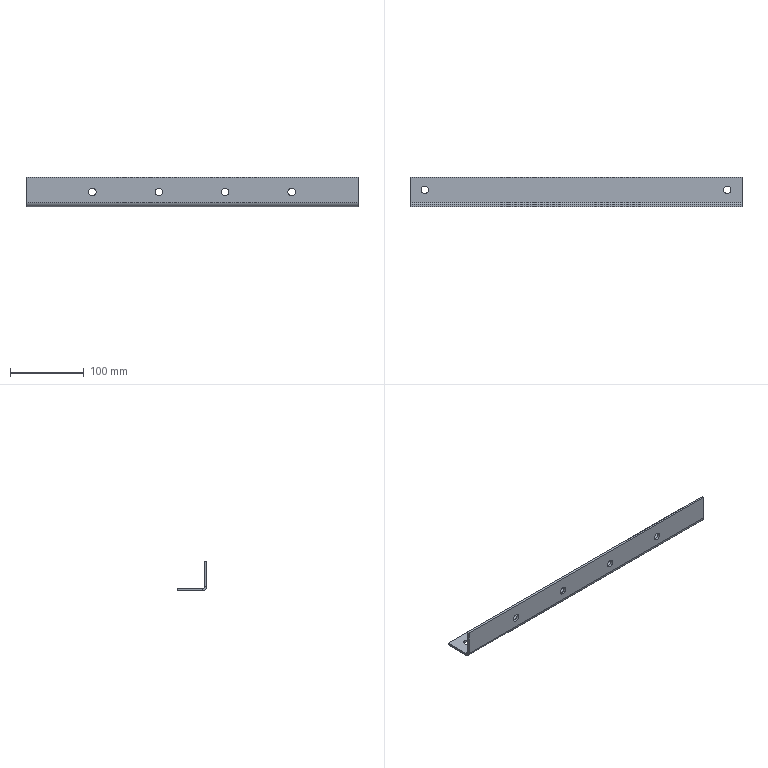Part | SolidWorks | features EdgeFlange 1, FlatPattern 1, ICE 1, SMBaseFlange 1, SheetMetal 1 | 1 solid | 26 faces | box 450 x 40 x 40 mm | volume 99929 mm3 | cylinder 14 | plane 12 | commonest cylinder face diameters 10 x12 6 x1 12 x1
STEP:
#1=CARTESIAN_POINT('',(-210.,23.,-20.));
#2=VERTEX_POINT('',#1);
#3=CARTESIAN_POINT('',(-200.,23.,-20.));
#4=VERTEX_POINT('',#3);
#5=CARTESIAN_POINT('',(-205.,23.,-20.));
#6=DIRECTION('',(0.,0.,1.));
#7=DIRECTION('',(0.,-1.,0.));
#8=AXIS2_PLACEMENT_3D('',#5,#6,#7);
#9=CIRCLE('',#8,5.);
#10=EDGE_CURVE('',#2,#4,#9,.T.);
#11=ORIENTED_EDGE('',*,*,#10,.F.);
#12=CARTESIAN_POINT('',(-210.,23.,-17.));
#13=VERTEX_POINT('',#12);
#14=CARTESIAN_POINT('',(-210.,23.,-27.));
#15=DIRECTION('',(0.,0.,1.));
#16=VECTOR('',#15,1000.);
#17=LINE('',#14,#16);
#18=EDGE_CURVE('',#2,#13,#17,.T.);
#19=ORIENTED_EDGE('',*,*,#18,.T.);
#20=CARTESIAN_POINT('',(-200.,23.,-17.));
#21=VERTEX_POINT('',#20);
#22=CARTESIAN_POINT('',(-205.,23.,-17.));
#23=DIRECTION('',(0.,0.,1.));
#24=DIRECTION('',(1.,0.,0.));
#25=AXIS2_PLACEMENT_3D('',#22,#23,#24);
#26=CIRCLE('',#25,5.);
#27=EDGE_CURVE('',#13,#21,#26,.T.);
#28=ORIENTED_EDGE('',*,*,#27,.T.);
#29=CARTESIAN_POINT('',(-200.,23.,-27.));
#30=DIRECTION('',(0.,0.,1.));
#31=VECTOR('',#30,1000.);
#32=LINE('',#29,#31);
#33=EDGE_CURVE('',#4,#21,#32,.T.);
#34=ORIENTED_EDGE('',*,*,#33,.F.);
#35=EDGE_LOOP('',(#11,#19,#28,#34));
#36=FACE_OUTER_BOUND('',#35,.T.);
#37=CARTESIAN_POINT('',(-205.,23.,-27.));
#38=DIRECTION('',(0.,0.,1.));
#39=DIRECTION('',(1.,0.,0.));
#40=AXIS2_PLACEMENT_3D('',#37,#38,#39);
#41=CYLINDRICAL_SURFACE('',#40,5.);
#42=ADVANCED_FACE('',(#36),#41,.F.);
#43=CARTESIAN_POINT('',(200.,23.,-20.));
#44=VERTEX_POINT('',#43);
#45=CARTESIAN_POINT('',(210.,23.,-20.));
#46=VERTEX_POINT('',#45);
#47=CARTESIAN_POINT('',(205.,23.,-20.));
#48=DIRECTION('',(0.,0.,1.));
#49=DIRECTION('',(0.,-1.,0.));
#50=AXIS2_PLACEMENT_3D('',#47,#48,#49);
#51=CIRCLE('',#50,5.);
#52=EDGE_CURVE('',#44,#46,#51,.T.);
#53=ORIENTED_EDGE('',*,*,#52,.F.);
#54=CARTESIAN_POINT('',(200.,23.,-17.));
#55=VERTEX_POINT('',#54);
#56=CARTESIAN_POINT('',(200.,23.,-27.));
#57=DIRECTION('',(0.,0.,1.));
#58=VECTOR('',#57,1000.);
#59=LINE('',#56,#58);
#60=EDGE_CURVE('',#44,#55,#59,.T.);
#61=ORIENTED_EDGE('',*,*,#60,.T.);
#62=CARTESIAN_POINT('',(210.,23.,-17.));
#63=VERTEX_POINT('',#62);
#64=CARTESIAN_POINT('',(205.,23.,-17.));
#65=DIRECTION('',(0.,0.,1.));
#66=DIRECTION('',(-1.,0.,0.));
#67=AXIS2_PLACEMENT_3D('',#64,#65,#66);
#68=CIRCLE('',#67,5.);
#69=EDGE_CURVE('',#55,#63,#68,.T.);
#70=ORIENTED_EDGE('',*,*,#69,.T.);
#71=CARTESIAN_POINT('',(210.,23.,-27.));
#72=DIRECTION('',(0.,0.,1.));
#73=VECTOR('',#72,1000.);
#74=LINE('',#71,#73);
#75=EDGE_CURVE('',#46,#63,#74,.T.);
#76=ORIENTED_EDGE('',*,*,#75,.F.);
#77=EDGE_LOOP('',(#53,#61,#70,#76));
#78=FACE_OUTER_BOUND('',#77,.T.);
#79=CARTESIAN_POINT('',(205.,23.,-27.));
#80=DIRECTION('',(0.,0.,1.));
#81=DIRECTION('',(1.,0.,0.));
#82=AXIS2_PLACEMENT_3D('',#79,#80,#81);
#83=CYLINDRICAL_SURFACE('',#82,5.);
#84=ADVANCED_FACE('',(#78),#83,.F.);
#85=CARTESIAN_POINT('',(135.,3.,-5.));
#86=VERTEX_POINT('',#85);
#87=CARTESIAN_POINT('',(135.,3.,5.));
#88=VERTEX_POINT('',#87);
#89=CARTESIAN_POINT('',(135.,3.,0.));
#90=DIRECTION('',(0.,1.,0.));
#91=DIRECTION('',(0.,0.,1.));
#92=AXIS2_PLACEMENT_3D('',#89,#90,#91);
#93=CIRCLE('',#92,5.);
#94=EDGE_CURVE('',#86,#88,#93,.T.);
#95=ORIENTED_EDGE('',*,*,#94,.T.);
#96=CARTESIAN_POINT('',(135.,0.,5.));
#97=VERTEX_POINT('',#96);
#98=CARTESIAN_POINT('',(135.,3.,5.));
#99=DIRECTION('',(0.,-1.,0.));
#100=VECTOR('',#99,1000.);
#101=LINE('',#98,#100);
#102=EDGE_CURVE('',#88,#97,#101,.T.);
#103=ORIENTED_EDGE('',*,*,#102,.T.);
#104=CARTESIAN_POINT('',(135.,0.,-5.));
#105=VERTEX_POINT('',#104);
#106=CARTESIAN_POINT('',(135.,0.,0.));
#107=DIRECTION('',(0.,1.,0.));
#108=DIRECTION('',(0.,0.,1.));
#109=AXIS2_PLACEMENT_3D('',#106,#107,#108);
#110=CIRCLE('',#109,5.);
#111=EDGE_CURVE('',#105,#97,#110,.T.);
#112=ORIENTED_EDGE('',*,*,#111,.F.);
#113=CARTESIAN_POINT('',(135.,3.,-5.));
#114=DIRECTION('',(0.,-1.,0.));
#115=VECTOR('',#114,1000.);
#116=LINE('',#113,#115);
#117=EDGE_CURVE('',#86,#105,#116,.T.);
#118=ORIENTED_EDGE('',*,*,#117,.F.);
#119=EDGE_LOOP('',(#95,#103,#112,#118));
#120=FACE_OUTER_BOUND('',#119,.T.);
#121=CARTESIAN_POINT('',(135.,3.,0.));
#122=DIRECTION('',(0.,-1.,0.));
#123=DIRECTION('',(0.,0.,-1.));
#124=AXIS2_PLACEMENT_3D('',#121,#122,#123);
#125=CYLINDRICAL_SURFACE('',#124,5.);
#126=ADVANCED_FACE('',(#120),#125,.F.);
#127=CARTESIAN_POINT('',(45.,3.,-5.));
#128=VERTEX_POINT('',#127);
#129=CARTESIAN_POINT('',(45.,3.,5.));
#130=VERTEX_POINT('',#129);
#131=CARTESIAN_POINT('',(45.,3.,0.));
#132=DIRECTION('',(0.,1.,0.));
#133=DIRECTION('',(0.,0.,1.));
#134=AXIS2_PLACEMENT_3D('',#131,#132,#133);
#135=CIRCLE('',#134,5.);
#136=EDGE_CURVE('',#128,#130,#135,.T.);
#137=ORIENTED_EDGE('',*,*,#136,.T.);
#138=CARTESIAN_POINT('',(45.,0.,5.));
#139=VERTEX_POINT('',#138);
#140=CARTESIAN_POINT('',(45.,3.,5.));
#141=DIRECTION('',(0.,-1.,0.));
#142=VECTOR('',#141,1000.);
#143=LINE('',#140,#142);
#144=EDGE_CURVE('',#130,#139,#143,.T.);
#145=ORIENTED_EDGE('',*,*,#144,.T.);
#146=CARTESIAN_POINT('',(45.,0.,-5.));
#147=VERTEX_POINT('',#146);
#148=CARTESIAN_POINT('',(45.,0.,0.));
#149=DIRECTION('',(0.,1.,0.));
#150=DIRECTION('',(0.,0.,1.));
#151=AXIS2_PLACEMENT_3D('',#148,#149,#150);
#152=CIRCLE('',#151,5.);
#153=EDGE_CURVE('',#147,#139,#152,.T.);
#154=ORIENTED_EDGE('',*,*,#153,.F.);
#155=CARTESIAN_POINT('',(45.,3.,-5.));
#156=DIRECTION('',(0.,-1.,0.));
#157=VECTOR('',#156,1000.);
#158=LINE('',#155,#157);
#159=EDGE_CURVE('',#128,#147,#158,.T.);
#160=ORIENTED_EDGE('',*,*,#159,.F.);
#161=EDGE_LOOP('',(#137,#145,#154,#160));
#162=FACE_OUTER_BOUND('',#161,.T.);
#163=CARTESIAN_POINT('',(45.,3.,0.));
#164=DIRECTION('',(0.,-1.,0.));
#165=DIRECTION('',(0.,0.,-1.));
#166=AXIS2_PLACEMENT_3D('',#163,#164,#165);
#167=CYLINDRICAL_SURFACE('',#166,5.);
#168=ADVANCED_FACE('',(#162),#167,.F.);
#169=CARTESIAN_POINT('',(-45.,3.,-5.));
#170=VERTEX_POINT('',#169);
#171=CARTESIAN_POINT('',(-45.,3.,5.));
#172=VERTEX_POINT('',#171);
#173=CARTESIAN_POINT('',(-45.,3.,0.));
#174=DIRECTION('',(0.,1.,0.));
#175=DIRECTION('',(0.,0.,1.));
#176=AXIS2_PLACEMENT_3D('',#173,#174,#175);
#177=CIRCLE('',#176,5.);
#178=EDGE_CURVE('',#170,#172,#177,.T.);
#179=ORIENTED_EDGE('',*,*,#178,.T.);
#180=CARTESIAN_POINT('',(-45.,0.,5.));
#181=VERTEX_POINT('',#180);
#182=CARTESIAN_POINT('',(-45.,3.,5.));
#183=DIRECTION('',(0.,-1.,0.));
#184=VECTOR('',#183,1000.);
#185=LINE('',#182,#184);
#186=EDGE_CURVE('',#172,#181,#185,.T.);
#187=ORIENTED_EDGE('',*,*,#186,.T.);
#188=CARTESIAN_POINT('',(-45.,0.,-5.));
#189=VERTEX_POINT('',#188);
#190=CARTESIAN_POINT('',(-45.,0.,0.));
#191=DIRECTION('',(0.,1.,0.));
#192=DIRECTION('',(0.,0.,1.));
#193=AXIS2_PLACEMENT_3D('',#190,#191,#192);
#194=CIRCLE('',#193,5.);
#195=EDGE_CURVE('',#189,#181,#194,.T.);
#196=ORIENTED_EDGE('',*,*,#195,.F.);
#197=CARTESIAN_POINT('',(-45.,3.,-5.));
#198=DIRECTION('',(0.,-1.,0.));
#199=VECTOR('',#198,1000.);
#200=LINE('',#197,#199);
#201=EDGE_CURVE('',#170,#189,#200,.T.);
#202=ORIENTED_EDGE('',*,*,#201,.F.);
#203=EDGE_LOOP('',(#179,#187,#196,#202));
#204=FACE_OUTER_BOUND('',#203,.T.);
#205=CARTESIAN_POINT('',(-45.,3.,0.));
#206=DIRECTION('',(0.,-1.,0.));
#207=DIRECTION('',(0.,0.,-1.));
#208=AXIS2_PLACEMENT_3D('',#205,#206,#207);
#209=CYLINDRICAL_SURFACE('',#208,5.);
#210=ADVANCED_FACE('',(#204),#209,.F.);
#211=CARTESIAN_POINT('',(-135.,3.,-5.));
#212=VERTEX_POINT('',#211);
#213=CARTESIAN_POINT('',(-135.,3.,5.));
#214=VERTEX_POINT('',#213);
#215=CARTESIAN_POINT('',(-135.,3.,0.));
#216=DIRECTION('',(0.,1.,0.));
#217=DIRECTION('',(0.,0.,1.));
#218=AXIS2_PLACEMENT_3D('',#215,#216,#217);
#219=CIRCLE('',#218,5.);
#220=EDGE_CURVE('',#212,#214,#219,.T.);
#221=ORIENTED_EDGE('',*,*,#220,.T.);
#222=CARTESIAN_POINT('',(-135.,0.,5.));
#223=VERTEX_POINT('',#222);
#224=CARTESIAN_POINT('',(-135.,3.,5.));
#225=DIRECTION('',(0.,-1.,0.));
#226=VECTOR('',#225,1000.);
#227=LINE('',#224,#226);
#228=EDGE_CURVE('',#214,#223,#227,.T.);
#229=ORIENTED_EDGE('',*,*,#228,.T.);
#230=CARTESIAN_POINT('',(-135.,0.,-5.));
#231=VERTEX_POINT('',#230);
#232=CARTESIAN_POINT('',(-135.,0.,0.));
#233=DIRECTION('',(0.,1.,0.));
#234=DIRECTION('',(0.,0.,1.));
#235=AXIS2_PLACEMENT_3D('',#232,#233,#234);
#236=CIRCLE('',#235,5.);
#237=EDGE_CURVE('',#231,#223,#236,.T.);
#238=ORIENTED_EDGE('',*,*,#237,.F.);
#239=CARTESIAN_POINT('',(-135.,3.,-5.));
#240=DIRECTION('',(0.,-1.,0.));
#241=VECTOR('',#240,1000.);
#242=LINE('',#239,#241);
#243=EDGE_CURVE('',#212,#231,#242,.T.);
#244=ORIENTED_EDGE('',*,*,#243,.F.);
#245=EDGE_LOOP('',(#221,#229,#238,#244));
#246=FACE_OUTER_BOUND('',#245,.T.);
#247=CARTESIAN_POINT('',(-135.,3.,0.));
#248=DIRECTION('',(0.,-1.,0.));
#249=DIRECTION('',(0.,0.,-1.));
#250=AXIS2_PLACEMENT_3D('',#247,#248,#249);
#251=CYLINDRICAL_SURFACE('',#250,5.);
#252=ADVANCED_FACE('',(#246),#251,.F.);
#253=ORIENTED_EDGE('',*,*,#136,.F.);
#254=CARTESIAN_POINT('',(45.,3.,0.));
#255=DIRECTION('',(0.,1.,0.));
#256=DIRECTION('',(0.,0.,1.));
#257=AXIS2_PLACEMENT_3D('',#254,#255,#256);
#258=CIRCLE('',#257,5.);
#259=EDGE_CURVE('',#130,#128,#258,.T.);
#260=ORIENTED_EDGE('',*,*,#259,.F.);
#261=EDGE_LOOP('',(#253,#260));
#262=FACE_BOUND('',#261,.T.);
#263=ORIENTED_EDGE('',*,*,#220,.F.);
#264=CARTESIAN_POINT('',(-135.,3.,0.));
#265=DIRECTION('',(0.,1.,0.));
#266=DIRECTION('',(0.,0.,1.));
#267=AXIS2_PLACEMENT_3D('',#264,#265,#266);
#268=CIRCLE('',#267,5.);
#269=EDGE_CURVE('',#214,#212,#268,.T.);
#270=ORIENTED_EDGE('',*,*,#269,.F.);
#271=EDGE_LOOP('',(#263,#270));
#272=FACE_BOUND('',#271,.T.);
#273=ORIENTED_EDGE('',*,*,#178,.F.);
#274=CARTESIAN_POINT('',(-45.,3.,0.));
#275=DIRECTION('',(0.,1.,0.));
#276=DIRECTION('',(0.,0.,1.));
#277=AXIS2_PLACEMENT_3D('',#274,#275,#276);
#278=CIRCLE('',#277,5.);
#279=EDGE_CURVE('',#172,#170,#278,.T.);
#280=ORIENTED_EDGE('',*,*,#279,.F.);
#281=EDGE_LOOP('',(#273,#280));
#282=FACE_BOUND('',#281,.T.);
#283=ORIENTED_EDGE('',*,*,#94,.F.);
#284=CARTESIAN_POINT('',(135.,3.,0.));
#285=DIRECTION('',(0.,1.,0.));
#286=DIRECTION('',(0.,0.,1.));
#287=AXIS2_PLACEMENT_3D('',#284,#285,#286);
#288=CIRCLE('',#287,5.);
#289=EDGE_CURVE('',#88,#86,#288,.T.);
#290=ORIENTED_EDGE('',*,*,#289,.F.);
#291=EDGE_LOOP('',(#283,#290));
#292=FACE_BOUND('',#291,.T.);
#293=CARTESIAN_POINT('',(225.,3.,20.));
#294=VERTEX_POINT('',#293);
#295=CARTESIAN_POINT('',(225.,3.,-14.));
#296=VERTEX_POINT('',#295);
#297=CARTESIAN_POINT('',(225.,3.,-20.));
#298=DIRECTION('',(0.,0.,-1.));
#299=VECTOR('',#298,1000.);
#300=LINE('',#297,#299);
#301=EDGE_CURVE('',#294,#296,#300,.T.);
#302=ORIENTED_EDGE('',*,*,#301,.T.);
#303=CARTESIAN_POINT('',(-225.,3.,-14.));
#304=VERTEX_POINT('',#303);
#305=CARTESIAN_POINT('',(-225.,3.,-14.));
#306=DIRECTION('',(1.,0.,0.));
#307=VECTOR('',#306,1000.);
#308=LINE('',#305,#307);
#309=EDGE_CURVE('',#304,#296,#308,.T.);
#310=ORIENTED_EDGE('',*,*,#309,.F.);
#311=CARTESIAN_POINT('',(-225.,3.,20.));
#312=VERTEX_POINT('',#311);
#313=CARTESIAN_POINT('',(-225.,3.,-20.));
#314=DIRECTION('',(0.,0.,1.));
#315=VECTOR('',#314,1000.);
#316=LINE('',#313,#315);
#317=EDGE_CURVE('',#304,#312,#316,.T.);
#318=ORIENTED_EDGE('',*,*,#317,.T.);
#319=CARTESIAN_POINT('',(-225.,3.,20.));
#320=DIRECTION('',(1.,0.,0.));
#321=VECTOR('',#320,1000.);
#322=LINE('',#319,#321);
#323=EDGE_CURVE('',#312,#294,#322,.T.);
#324=ORIENTED_EDGE('',*,*,#323,.T.);
#325=EDGE_LOOP('',(#302,#310,#318,#324));
#326=FACE_OUTER_BOUND('',#325,.T.);
#327=CARTESIAN_POINT('',(0.,3.,0.));
#328=DIRECTION('',(0.,1.,0.));
#329=DIRECTION('',(0.,0.,1.));
#330=AXIS2_PLACEMENT_3D('',#327,#328,#329);
#331=PLANE('',#330);
#332=ADVANCED_FACE('',(#262,#272,#282,#292,#326),#331,.T.);
#333=ORIENTED_EDGE('',*,*,#111,.T.);
#334=CARTESIAN_POINT('',(135.,0.,0.));
#335=DIRECTION('',(0.,1.,0.));
#336=DIRECTION('',(0.,0.,1.));
#337=AXIS2_PLACEMENT_3D('',#334,#335,#336);
#338=CIRCLE('',#337,5.);
#339=EDGE_CURVE('',#97,#105,#338,.T.);
#340=ORIENTED_EDGE('',*,*,#339,.T.);
#341=EDGE_LOOP('',(#333,#340));
#342=FACE_BOUND('',#341,.T.);
#343=ORIENTED_EDGE('',*,*,#153,.T.);
#344=CARTESIAN_POINT('',(45.,0.,0.));
#345=DIRECTION('',(0.,1.,0.));
#346=DIRECTION('',(0.,0.,1.));
#347=AXIS2_PLACEMENT_3D('',#344,#345,#346);
#348=CIRCLE('',#347,5.);
#349=EDGE_CURVE('',#139,#147,#348,.T.);
#350=ORIENTED_EDGE('',*,*,#349,.T.);
#351=EDGE_LOOP('',(#343,#350));
#352=FACE_BOUND('',#351,.T.);
#353=ORIENTED_EDGE('',*,*,#195,.T.);
#354=CARTESIAN_POINT('',(-45.,0.,0.));
#355=DIRECTION('',(0.,1.,0.));
#356=DIRECTION('',(0.,0.,1.));
#357=AXIS2_PLACEMENT_3D('',#354,#355,#356);
#358=CIRCLE('',#357,5.);
#359=EDGE_CURVE('',#181,#189,#358,.T.);
#360=ORIENTED_EDGE('',*,*,#359,.T.);
#361=EDGE_LOOP('',(#353,#360));
#362=FACE_BOUND('',#361,.T.);
#363=ORIENTED_EDGE('',*,*,#237,.T.);
#364=CARTESIAN_POINT('',(-135.,0.,0.));
#365=DIRECTION('',(0.,1.,0.));
#366=DIRECTION('',(0.,0.,1.));
#367=AXIS2_PLACEMENT_3D('',#364,#365,#366);
#368=CIRCLE('',#367,5.);
#369=EDGE_CURVE('',#223,#231,#368,.T.);
#370=ORIENTED_EDGE('',*,*,#369,.T.);
#371=EDGE_LOOP('',(#363,#370));
#372=FACE_BOUND('',#371,.T.);
#373=CARTESIAN_POINT('',(-225.,0.,-14.));
#374=VERTEX_POINT('',#373);
#375=CARTESIAN_POINT('',(225.,0.,-14.));
#376=VERTEX_POINT('',#375);
#377=CARTESIAN_POINT('',(-225.,0.,-14.));
#378=DIRECTION('',(1.,0.,0.));
#379=VECTOR('',#378,1000.);
#380=LINE('',#377,#379);
#381=EDGE_CURVE('',#374,#376,#380,.T.);
#382=ORIENTED_EDGE('',*,*,#381,.T.);
#383=CARTESIAN_POINT('',(225.,0.,20.));
#384=VERTEX_POINT('',#383);
#385=CARTESIAN_POINT('',(225.,0.,-20.));
#386=DIRECTION('',(0.,0.,-1.));
#387=VECTOR('',#386,1000.);
#388=LINE('',#385,#387);
#389=EDGE_CURVE('',#384,#376,#388,.T.);
#390=ORIENTED_EDGE('',*,*,#389,.F.);
#391=CARTESIAN_POINT('',(-225.,0.,20.));
#392=VERTEX_POINT('',#391);
#393=CARTESIAN_POINT('',(-225.,0.,20.));
#394=DIRECTION('',(1.,0.,0.));
#395=VECTOR('',#394,1000.);
#396=LINE('',#393,#395);
#397=EDGE_CURVE('',#392,#384,#396,.T.);
#398=ORIENTED_EDGE('',*,*,#397,.F.);
#399=CARTESIAN_POINT('',(-225.,0.,-20.));
#400=DIRECTION('',(0.,0.,1.));
#401=VECTOR('',#400,1000.);
#402=LINE('',#399,#401);
#403=EDGE_CURVE('',#374,#392,#402,.T.);
#404=ORIENTED_EDGE('',*,*,#403,.F.);
#405=EDGE_LOOP('',(#382,#390,#398,#404));
#406=FACE_OUTER_BOUND('',#405,.T.);
#407=CARTESIAN_POINT('',(0.,0.,0.));
#408=DIRECTION('',(0.,1.,0.));
#409=DIRECTION('',(0.,0.,1.));
#410=AXIS2_PLACEMENT_3D('',#407,#408,#409);
#411=PLANE('',#410);
#412=ADVANCED_FACE('',(#342,#352,#362,#372,#406),#411,.F.);
#413=CARTESIAN_POINT('',(225.,3.,-14.));
#414=DIRECTION('',(0.,-1.,0.));
#415=VECTOR('',#414,1000.);
#416=LINE('',#413,#415);
#417=EDGE_CURVE('',#296,#376,#416,.T.);
#418=ORIENTED_EDGE('',*,*,#417,.F.);
#419=ORIENTED_EDGE('',*,*,#301,.F.);
#420=CARTESIAN_POINT('',(225.,3.,20.));
#421=DIRECTION('',(0.,-1.,0.));
#422=VECTOR('',#421,1000.);
#423=LINE('',#420,#422);
#424=EDGE_CURVE('',#294,#384,#423,.T.);
#425=ORIENTED_EDGE('',*,*,#424,.T.);
#426=ORIENTED_EDGE('',*,*,#389,.T.);
#427=EDGE_LOOP('',(#418,#419,#425,#426));
#428=FACE_OUTER_BOUND('',#427,.T.);
#429=CARTESIAN_POINT('',(225.,3.,-20.));
#430=DIRECTION('',(-1.,0.,0.));
#431=DIRECTION('',(0.,0.,1.));
#432=AXIS2_PLACEMENT_3D('',#429,#430,#431);
#433=PLANE('',#432);
#434=ADVANCED_FACE('',(#428),#433,.F.);
#435=CARTESIAN_POINT('',(-225.,3.,-14.));
#436=DIRECTION('',(0.,-1.,0.));
#437=VECTOR('',#436,1000.);
#438=LINE('',#435,#437);
#439=EDGE_CURVE('',#304,#374,#438,.T.);
#440=ORIENTED_EDGE('',*,*,#439,.T.);
#441=ORIENTED_EDGE('',*,*,#403,.T.);
#442=CARTESIAN_POINT('',(-225.,3.,20.));
#443=DIRECTION('',(0.,-1.,0.));
#444=VECTOR('',#443,1000.);
#445=LINE('',#442,#444);
#446=EDGE_CURVE('',#312,#392,#445,.T.);
#447=ORIENTED_EDGE('',*,*,#446,.F.);
#448=ORIENTED_EDGE('',*,*,#317,.F.);
#449=EDGE_LOOP('',(#440,#441,#447,#448));
#450=FACE_OUTER_BOUND('',#449,.T.);
#451=CARTESIAN_POINT('',(-225.,3.,-20.));
#452=DIRECTION('',(1.,0.,0.));
#453=DIRECTION('',(0.,0.,-1.));
#454=AXIS2_PLACEMENT_3D('',#451,#452,#453);
#455=PLANE('',#454);
#456=ADVANCED_FACE('',(#450),#455,.F.);
#457=ORIENTED_EDGE('',*,*,#397,.T.);
#458=ORIENTED_EDGE('',*,*,#424,.F.);
#459=ORIENTED_EDGE('',*,*,#323,.F.);
#460=ORIENTED_EDGE('',*,*,#446,.T.);
#461=EDGE_LOOP('',(#457,#458,#459,#460));
#462=FACE_OUTER_BOUND('',#461,.T.);
#463=CARTESIAN_POINT('',(-225.,3.,20.));
#464=DIRECTION('',(0.,0.,-1.));
#465=DIRECTION('',(-1.,0.,0.));
#466=AXIS2_PLACEMENT_3D('',#463,#464,#465);
#467=PLANE('',#466);
#468=ADVANCED_FACE('',(#462),#467,.F.);
#469=ORIENTED_EDGE('',*,*,#228,.F.);
#470=ORIENTED_EDGE('',*,*,#269,.T.);
#471=ORIENTED_EDGE('',*,*,#243,.T.);
#472=ORIENTED_EDGE('',*,*,#369,.F.);
#473=EDGE_LOOP('',(#469,#470,#471,#472));
#474=FACE_OUTER_BOUND('',#473,.T.);
#475=CARTESIAN_POINT('',(-135.,3.,0.));
#476=DIRECTION('',(0.,-1.,0.));
#477=DIRECTION('',(0.,0.,-1.));
#478=AXIS2_PLACEMENT_3D('',#475,#476,#477);
#479=CYLINDRICAL_SURFACE('',#478,5.);
#480=ADVANCED_FACE('',(#474),#479,.F.);
#481=ORIENTED_EDGE('',*,*,#186,.F.);
#482=ORIENTED_EDGE('',*,*,#279,.T.);
#483=ORIENTED_EDGE('',*,*,#201,.T.);
#484=ORIENTED_EDGE('',*,*,#359,.F.);
#485=EDGE_LOOP('',(#481,#482,#483,#484));
#486=FACE_OUTER_BOUND('',#485,.T.);
#487=CARTESIAN_POINT('',(-45.,3.,0.));
#488=DIRECTION('',(0.,-1.,0.));
#489=DIRECTION('',(0.,0.,-1.));
#490=AXIS2_PLACEMENT_3D('',#487,#488,#489);
#491=CYLINDRICAL_SURFACE('',#490,5.);
#492=ADVANCED_FACE('',(#486),#491,.F.);
#493=ORIENTED_EDGE('',*,*,#144,.F.);
#494=ORIENTED_EDGE('',*,*,#259,.T.);
#495=ORIENTED_EDGE('',*,*,#159,.T.);
#496=ORIENTED_EDGE('',*,*,#349,.F.);
#497=EDGE_LOOP('',(#493,#494,#495,#496));
#498=FACE_OUTER_BOUND('',#497,.T.);
#499=CARTESIAN_POINT('',(45.,3.,0.));
#500=DIRECTION('',(0.,-1.,0.));
#501=DIRECTION('',(0.,0.,-1.));
#502=AXIS2_PLACEMENT_3D('',#499,#500,#501);
#503=CYLINDRICAL_SURFACE('',#502,5.);
#504=ADVANCED_FACE('',(#498),#503,.F.);
#505=ORIENTED_EDGE('',*,*,#102,.F.);
#506=ORIENTED_EDGE('',*,*,#289,.T.);
#507=ORIENTED_EDGE('',*,*,#117,.T.);
#508=ORIENTED_EDGE('',*,*,#339,.F.);
#509=EDGE_LOOP('',(#505,#506,#507,#508));
#510=FACE_OUTER_BOUND('',#509,.T.);
#511=CARTESIAN_POINT('',(135.,3.,0.));
#512=DIRECTION('',(0.,-1.,0.));
#513=DIRECTION('',(0.,0.,-1.));
#514=AXIS2_PLACEMENT_3D('',#511,#512,#513);
#515=CYLINDRICAL_SURFACE('',#514,5.);
#516=ADVANCED_FACE('',(#510),#515,.F.);
#517=CARTESIAN_POINT('',(225.,6.,-17.));
#518=VERTEX_POINT('',#517);
#519=CARTESIAN_POINT('',(225.,6.,-20.));
#520=VERTEX_POINT('',#519);
#521=CARTESIAN_POINT('',(225.,6.,-20.));
#522=DIRECTION('',(0.,0.,-1.));
#523=VECTOR('',#522,1000.);
#524=LINE('',#521,#523);
#525=EDGE_CURVE('',#518,#520,#524,.T.);
#526=ORIENTED_EDGE('',*,*,#525,.F.);
#527=CARTESIAN_POINT('',(225.,6.,-14.));
#528=DIRECTION('',(1.,0.,0.));
#529=DIRECTION('',(0.,0.,1.));
#530=AXIS2_PLACEMENT_3D('',#527,#528,#529);
#531=CIRCLE('',#530,3.);
#532=EDGE_CURVE('',#296,#518,#531,.T.);
#533=ORIENTED_EDGE('',*,*,#532,.F.);
#534=ORIENTED_EDGE('',*,*,#417,.T.);
#535=CARTESIAN_POINT('',(225.,6.,-14.));
#536=DIRECTION('',(1.,0.,0.));
#537=DIRECTION('',(0.,0.,1.));
#538=AXIS2_PLACEMENT_3D('',#535,#536,#537);
#539=CIRCLE('',#538,6.);
#540=EDGE_CURVE('',#376,#520,#539,.T.);
#541=ORIENTED_EDGE('',*,*,#540,.T.);
#542=EDGE_LOOP('',(#526,#533,#534,#541));
#543=FACE_OUTER_BOUND('',#542,.T.);
#544=CARTESIAN_POINT('',(225.,6.,-14.));
#545=DIRECTION('',(1.,0.,0.));
#546=DIRECTION('',(0.,0.,-1.));
#547=AXIS2_PLACEMENT_3D('',#544,#545,#546);
#548=PLANE('',#547);
#549=ADVANCED_FACE('',(#543),#548,.T.);
#550=CARTESIAN_POINT('',(-225.,6.,-17.));
#551=VERTEX_POINT('',#550);
#552=CARTESIAN_POINT('',(-225.,6.,-14.));
#553=DIRECTION('',(-1.,0.,0.));
#554=DIRECTION('',(0.,0.,1.));
#555=AXIS2_PLACEMENT_3D('',#552,#553,#554);
#556=CIRCLE('',#555,3.);
#557=EDGE_CURVE('',#551,#304,#556,.T.);
#558=ORIENTED_EDGE('',*,*,#557,.F.);
#559=CARTESIAN_POINT('',(-225.,6.,-20.));
#560=VERTEX_POINT('',#559);
#561=CARTESIAN_POINT('',(-225.,6.,-17.));
#562=DIRECTION('',(0.,0.,-1.));
#563=VECTOR('',#562,1000.);
#564=LINE('',#561,#563);
#565=EDGE_CURVE('',#551,#560,#564,.T.);
#566=ORIENTED_EDGE('',*,*,#565,.T.);
#567=CARTESIAN_POINT('',(-225.,6.,-14.));
#568=DIRECTION('',(-1.,0.,0.));
#569=DIRECTION('',(0.,0.,1.));
#570=AXIS2_PLACEMENT_3D('',#567,#568,#569);
#571=CIRCLE('',#570,6.);
#572=EDGE_CURVE('',#560,#374,#571,.T.);
#573=ORIENTED_EDGE('',*,*,#572,.T.);
#574=ORIENTED_EDGE('',*,*,#439,.F.);
#575=EDGE_LOOP('',(#558,#566,#573,#574));
#576=FACE_OUTER_BOUND('',#575,.T.);
#577=CARTESIAN_POINT('',(-225.,6.,-14.));
#578=DIRECTION('',(1.,0.,0.));
#579=DIRECTION('',(0.,0.,-1.));
#580=AXIS2_PLACEMENT_3D('',#577,#578,#579);
#581=PLANE('',#580);
#582=ADVANCED_FACE('',(#576),#581,.F.);
#583=ORIENTED_EDGE('',*,*,#381,.F.);
#584=ORIENTED_EDGE('',*,*,#572,.F.);
#585=CARTESIAN_POINT('',(225.,6.,-20.));
#586=DIRECTION('',(1.,0.,0.));
#587=VECTOR('',#586,1000.);
#588=LINE('',#585,#587);
#589=EDGE_CURVE('',#560,#520,#588,.T.);
#590=ORIENTED_EDGE('',*,*,#589,.T.);
#591=ORIENTED_EDGE('',*,*,#540,.F.);
#592=EDGE_LOOP('',(#583,#584,#590,#591));
#593=FACE_OUTER_BOUND('',#592,.T.);
#594=CARTESIAN_POINT('',(-225.,6.,-14.));
#595=DIRECTION('',(-1.,0.,0.));
#596=DIRECTION('',(0.,0.,-1.));
#597=AXIS2_PLACEMENT_3D('',#594,#595,#596);
#598=CYLINDRICAL_SURFACE('',#597,6.);
#599=ADVANCED_FACE('',(#593),#598,.T.);
#600=ORIENTED_EDGE('',*,*,#309,.T.);
#601=ORIENTED_EDGE('',*,*,#532,.T.);
#602=CARTESIAN_POINT('',(225.,6.,-17.));
#603=DIRECTION('',(-1.,0.,0.));
#604=VECTOR('',#603,1000.);
#605=LINE('',#602,#604);
#606=EDGE_CURVE('',#518,#551,#605,.T.);
#607=ORIENTED_EDGE('',*,*,#606,.T.);
#608=ORIENTED_EDGE('',*,*,#557,.T.);
#609=EDGE_LOOP('',(#600,#601,#607,#608));
#610=FACE_OUTER_BOUND('',#609,.T.);
#611=CARTESIAN_POINT('',(-225.,6.,-14.));
#612=DIRECTION('',(-1.,0.,0.));
#613=DIRECTION('',(0.,0.,-1.));
#614=AXIS2_PLACEMENT_3D('',#611,#612,#613);
#615=CYLINDRICAL_SURFACE('',#614,3.);
#616=ADVANCED_FACE('',(#610),#615,.F.);
#617=ORIENTED_EDGE('',*,*,#525,.T.);
#618=CARTESIAN_POINT('',(225.,40.,-20.));
#619=VERTEX_POINT('',#618);
#620=CARTESIAN_POINT('',(225.,0.,-20.));
#621=DIRECTION('',(0.,-1.,0.));
#622=VECTOR('',#621,1000.);
#623=LINE('',#620,#622);
#624=EDGE_CURVE('',#619,#520,#623,.T.);
#625=ORIENTED_EDGE('',*,*,#624,.F.);
#626=CARTESIAN_POINT('',(225.,40.,-17.));
#627=VERTEX_POINT('',#626);
#628=CARTESIAN_POINT('',(225.,40.,-20.));
#629=DIRECTION('',(0.,0.,1.));
#630=VECTOR('',#629,1000.);
#631=LINE('',#628,#630);
#632=EDGE_CURVE('',#619,#627,#631,.T.);
#633=ORIENTED_EDGE('',*,*,#632,.T.);
#634=CARTESIAN_POINT('',(225.,3.,-17.));
#635=DIRECTION('',(0.,-1.,0.));
#636=VECTOR('',#635,1000.);
#637=LINE('',#634,#636);
#638=EDGE_CURVE('',#627,#518,#637,.T.);
#639=ORIENTED_EDGE('',*,*,#638,.T.);
#640=EDGE_LOOP('',(#617,#625,#633,#639));
#641=FACE_OUTER_BOUND('',#640,.T.);
#642=CARTESIAN_POINT('',(225.,3.,-20.));
#643=DIRECTION('',(-1.,0.,0.));
#644=DIRECTION('',(0.,0.,1.));
#645=AXIS2_PLACEMENT_3D('',#642,#643,#644);
#646=PLANE('',#645);
#647=ADVANCED_FACE('',(#641),#646,.F.);
#648=ORIENTED_EDGE('',*,*,#565,.F.);
#649=CARTESIAN_POINT('',(-225.,40.,-17.));
#650=VERTEX_POINT('',#649);
#651=CARTESIAN_POINT('',(-225.,40.,-17.));
#652=DIRECTION('',(0.,1.,0.));
#653=VECTOR('',#652,1000.);
#654=LINE('',#651,#653);
#655=EDGE_CURVE('',#551,#650,#654,.T.);
#656=ORIENTED_EDGE('',*,*,#655,.T.);
#657=CARTESIAN_POINT('',(-225.,40.,-20.));
#658=VERTEX_POINT('',#657);
#659=CARTESIAN_POINT('',(-225.,40.,-20.));
#660=DIRECTION('',(0.,0.,1.));
#661=VECTOR('',#660,1000.);
#662=LINE('',#659,#661);
#663=EDGE_CURVE('',#658,#650,#662,.T.);
#664=ORIENTED_EDGE('',*,*,#663,.F.);
#665=CARTESIAN_POINT('',(-225.,0.,-20.));
#666=DIRECTION('',(0.,1.,0.));
#667=VECTOR('',#666,1000.);
#668=LINE('',#665,#667);
#669=EDGE_CURVE('',#560,#658,#668,.T.);
#670=ORIENTED_EDGE('',*,*,#669,.F.);
#671=EDGE_LOOP('',(#648,#656,#664,#670));
#672=FACE_OUTER_BOUND('',#671,.T.);
#673=CARTESIAN_POINT('',(-225.,40.,-20.));
#674=DIRECTION('',(1.,0.,0.));
#675=DIRECTION('',(0.,0.,-1.));
#676=AXIS2_PLACEMENT_3D('',#673,#674,#675);
#677=PLANE('',#676);
#678=ADVANCED_FACE('',(#672),#677,.F.);
#679=CARTESIAN_POINT('',(-205.,23.,-20.));
#680=DIRECTION('',(0.,0.,1.));
#681=DIRECTION('',(0.,-1.,0.));
#682=AXIS2_PLACEMENT_3D('',#679,#680,#681);
#683=CIRCLE('',#682,5.);
#684=EDGE_CURVE('',#4,#2,#683,.T.);
#685=ORIENTED_EDGE('',*,*,#684,.T.);
#686=ORIENTED_EDGE('',*,*,#10,.T.);
#687=EDGE_LOOP('',(#685,#686));
#688=FACE_BOUND('',#687,.T.);
#689=CARTESIAN_POINT('',(205.,23.,-20.));
#690=DIRECTION('',(0.,0.,1.));
#691=DIRECTION('',(0.,-1.,0.));
#692=AXIS2_PLACEMENT_3D('',#689,#690,#691);
#693=CIRCLE('',#692,5.);
#694=EDGE_CURVE('',#46,#44,#693,.T.);
#695=ORIENTED_EDGE('',*,*,#694,.T.);
#696=ORIENTED_EDGE('',*,*,#52,.T.);
#697=EDGE_LOOP('',(#695,#696));
#698=FACE_BOUND('',#697,.T.);
#699=ORIENTED_EDGE('',*,*,#589,.F.);
#700=ORIENTED_EDGE('',*,*,#669,.T.);
#701=CARTESIAN_POINT('',(0.,40.,-20.));
#702=DIRECTION('',(1.,0.,0.));
#703=VECTOR('',#702,1000.);
#704=LINE('',#701,#703);
#705=EDGE_CURVE('',#658,#619,#704,.T.);
#706=ORIENTED_EDGE('',*,*,#705,.T.);
#707=ORIENTED_EDGE('',*,*,#624,.T.);
#708=EDGE_LOOP('',(#699,#700,#706,#707));
#709=FACE_OUTER_BOUND('',#708,.T.);
#710=CARTESIAN_POINT('',(0.,0.,-20.));
#711=DIRECTION('',(0.,0.,1.));
#712=DIRECTION('',(0.,-1.,0.));
#713=AXIS2_PLACEMENT_3D('',#710,#711,#712);
#714=PLANE('',#713);
#715=ADVANCED_FACE('',(#688,#698,#709),#714,.F.);
#716=CARTESIAN_POINT('',(-205.,23.,-17.));
#717=DIRECTION('',(0.,0.,1.));
#718=DIRECTION('',(1.,0.,0.));
#719=AXIS2_PLACEMENT_3D('',#716,#717,#718);
#720=CIRCLE('',#719,5.);
#721=EDGE_CURVE('',#21,#13,#720,.T.);
#722=ORIENTED_EDGE('',*,*,#721,.F.);
#723=ORIENTED_EDGE('',*,*,#27,.F.);
#724=EDGE_LOOP('',(#722,#723));
#725=FACE_BOUND('',#724,.T.);
#726=CARTESIAN_POINT('',(205.,23.,-17.));
#727=DIRECTION('',(0.,0.,1.));
#728=DIRECTION('',(-1.,0.,0.));
#729=AXIS2_PLACEMENT_3D('',#726,#727,#728);
#730=CIRCLE('',#729,5.);
#731=EDGE_CURVE('',#63,#55,#730,.T.);
#732=ORIENTED_EDGE('',*,*,#731,.F.);
#733=ORIENTED_EDGE('',*,*,#69,.F.);
#734=EDGE_LOOP('',(#732,#733));
#735=FACE_BOUND('',#734,.T.);
#736=ORIENTED_EDGE('',*,*,#655,.F.);
#737=ORIENTED_EDGE('',*,*,#606,.F.);
#738=ORIENTED_EDGE('',*,*,#638,.F.);
#739=CARTESIAN_POINT('',(225.,40.,-17.));
#740=DIRECTION('',(1.,0.,0.));
#741=VECTOR('',#740,1000.);
#742=LINE('',#739,#741);
#743=EDGE_CURVE('',#650,#627,#742,.T.);
#744=ORIENTED_EDGE('',*,*,#743,.F.);
#745=EDGE_LOOP('',(#736,#737,#738,#744));
#746=FACE_OUTER_BOUND('',#745,.T.);
#747=CARTESIAN_POINT('',(0.,0.,-17.));
#748=DIRECTION('',(0.,0.,1.));
#749=DIRECTION('',(0.,-1.,0.));
#750=AXIS2_PLACEMENT_3D('',#747,#748,#749);
#751=PLANE('',#750);
#752=ADVANCED_FACE('',(#725,#735,#746),#751,.T.);
#753=ORIENTED_EDGE('',*,*,#743,.T.);
#754=ORIENTED_EDGE('',*,*,#632,.F.);
#755=ORIENTED_EDGE('',*,*,#705,.F.);
#756=ORIENTED_EDGE('',*,*,#663,.T.);
#757=EDGE_LOOP('',(#753,#754,#755,#756));
#758=FACE_OUTER_BOUND('',#757,.T.);
#759=CARTESIAN_POINT('',(225.,40.,-20.));
#760=DIRECTION('',(0.,-1.,0.));
#761=DIRECTION('',(0.,0.,-1.));
#762=AXIS2_PLACEMENT_3D('',#759,#760,#761);
#763=PLANE('',#762);
#764=ADVANCED_FACE('',(#758),#763,.F.);
#765=ORIENTED_EDGE('',*,*,#60,.F.);
#766=ORIENTED_EDGE('',*,*,#694,.F.);
#767=ORIENTED_EDGE('',*,*,#75,.T.);
#768=ORIENTED_EDGE('',*,*,#731,.T.);
#769=EDGE_LOOP('',(#765,#766,#767,#768));
#770=FACE_OUTER_BOUND('',#769,.T.);
#771=CARTESIAN_POINT('',(205.,23.,-27.));
#772=DIRECTION('',(0.,0.,1.));
#773=DIRECTION('',(1.,0.,0.));
#774=AXIS2_PLACEMENT_3D('',#771,#772,#773);
#775=CYLINDRICAL_SURFACE('',#774,5.);
#776=ADVANCED_FACE('',(#770),#775,.F.);
#777=ORIENTED_EDGE('',*,*,#18,.F.);
#778=ORIENTED_EDGE('',*,*,#684,.F.);
#779=ORIENTED_EDGE('',*,*,#33,.T.);
#780=ORIENTED_EDGE('',*,*,#721,.T.);
#781=EDGE_LOOP('',(#777,#778,#779,#780));
#782=FACE_OUTER_BOUND('',#781,.T.);
#783=CARTESIAN_POINT('',(-205.,23.,-27.));
#784=DIRECTION('',(0.,0.,1.));
#785=DIRECTION('',(1.,0.,0.));
#786=AXIS2_PLACEMENT_3D('',#783,#784,#785);
#787=CYLINDRICAL_SURFACE('',#786,5.);
#788=ADVANCED_FACE('',(#782),#787,.F.);
#789=CLOSED_SHELL('',(#42,#84,#126,#168,#210,#252,#332,#412,#434,#456,#468,#480,#492,#504,#516,#549,#582,#599,#616,#647,#678,#715,#752,#764,#776,#788));
#790=MANIFOLD_SOLID_BREP('',#789);
#791=CARTESIAN_POINT('',(0.,0.,0.));
#792=DIRECTION('',(0.,0.,1.));
#793=DIRECTION('',(1.,0.,0.));
#794=AXIS2_PLACEMENT_3D('',#791,#792,#793);
#795=(LENGTH_UNIT()NAMED_UNIT(*)SI_UNIT(.MILLI.,.METRE.));
#796=UNCERTAINTY_MEASURE_WITH_UNIT(LENGTH_MEASURE(0.00001),#795,'','');
#797=(NAMED_UNIT(*)PLANE_ANGLE_UNIT()SI_UNIT($,.RADIAN.));
#798=(NAMED_UNIT(*)SI_UNIT($,.STERADIAN.)SOLID_ANGLE_UNIT());
#799=(GEOMETRIC_REPRESENTATION_CONTEXT(3)GLOBAL_UNCERTAINTY_ASSIGNED_CONTEXT((#796))GLOBAL_UNIT_ASSIGNED_CONTEXT((#795,#797,#798))REPRESENTATION_CONTEXT('',''));
#800=ADVANCED_BREP_SHAPE_REPRESENTATION('',(#790,#794),#799);